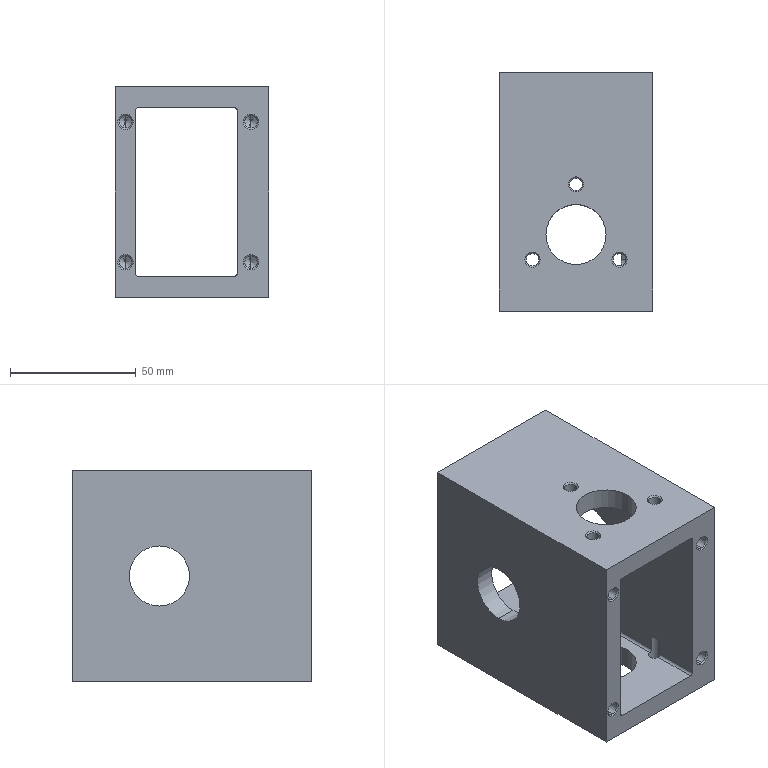Part | SolidWorks | features HoleWzd 4, ICE 4, Extrusion 1, Fillet 1, MirrorPattern 1 | 1 solid | 98 faces | box 61 x 95 x 84 mm | volume 198920 mm3 | cone 47 | cylinder 41 | plane 10 | commonest cylinder face diameters 5 x20 4.2 x8 24 x6 2 x5 40 x2